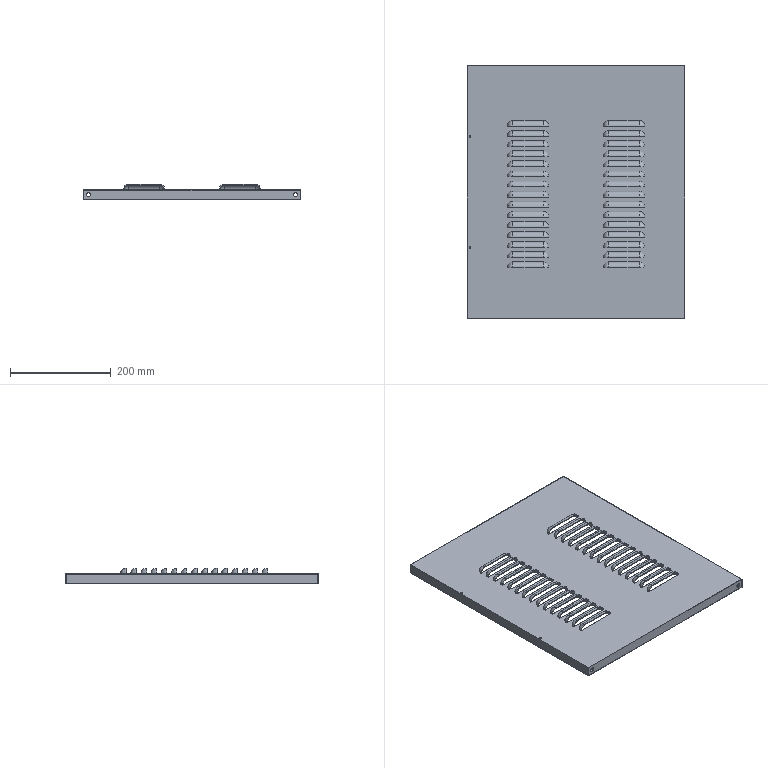Part | SolidWorks | features ICE 10, LPattern 4, MirrorPattern 3, HoleWzd 2, 3DProfileFeature 1, Chamfer 1, Extrusion 1, Fillet 1, Revolution 1, Shell 1 | 1 solid | 276 faces | box 430 x 500 x 30.5 mm | volume 310221 mm3 | sphere 120 | cylinder 80 | plane 76 | commonest cylinder face diameters 20 x30 23 x30 3.3 x12 8 x8